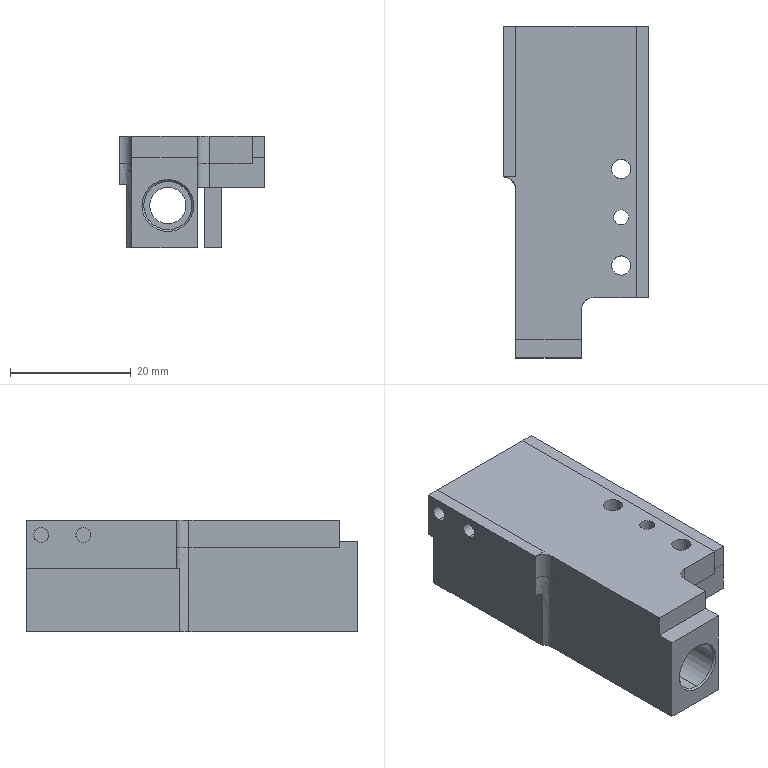NC program | NX | posted with a generic post | part box 24.15 x 55 x 18.5 mm
Lines 1748 to 2652 of 2652:
(CAVITY_MILL_COPY_COPY , TOOL : D3)
N3464 T03 M6
N3466 G54
N3468 G17 G0 G90 X18.9 Y17.954 B0. C0. S9500 M3
N3470 G43 Z30. H3
N3472 Z-0.2
N3474 G94 G1 X19. Y18.011 F1000.
N3476 G3 X19.5 Y18.877 R1.
N3478 G1 Y19.112 F1200.
N3480 G2 X20.919 Y20.573 R1.5
N3482 G1 X20.838 Y20.575
N3484 X17.928
N3486 G3 X17.062 Y20.075 R1.
N3488 G1 X17.005 Y19.975
N3490 G0 X18.9 Y17.954 Z-0.4
N3492 G1 X19. Y18.011 F1000.
N3494 G3 X19.5 Y18.877 R1.
N3496 G1 Y19.112 F1200.
N3498 G2 X20.919 Y20.573 R1.5
N3500 G1 X20.838 Y20.575
N3502 X17.928
N3504 G3 X17.062 Y20.075 R1.
N3506 G1 X17.005 Y19.975
N3508 G0 X18.9 Y17.954 Z-0.6
N3510 G1 X19. Y18.011 F1000.
N3512 G3 X19.5 Y18.877 R1.
N3514 G1 Y19.112 F1200.
N3516 G2 X20.919 Y20.573 R1.5
N3518 G1 X20.838 Y20.575
N3520 X17.928
N3522 G3 X17.062 Y20.075 R1.
N3524 G1 X17.005 Y19.975
N3526 G0 X18.9 Y17.954 Z-0.8
N3528 G1 X19. Y18.011 F1000.
N3530 G3 X19.5 Y18.877 R1.
N3532 G1 Y19.112 F1200.
N3534 G2 X20.919 Y20.573 R1.5
N3536 G1 X20.838 Y20.575
N3538 X17.928
N3540 G3 X17.062 Y20.075 R1.
N3542 G1 X17.005 Y19.975
N3544 G0 X18.9 Y17.954 Z-1.
N3546 G1 X19. Y18.011 F1000.
N3548 G3 X19.5 Y18.877 R1.
N3550 G1 Y19.112 F1200.
N3552 G2 X20.919 Y20.573 R1.5
N3554 G1 X20.838 Y20.575
N3556 X17.928
N3558 G3 X17.062 Y20.075 R1.
N3560 G1 X17.005 Y19.975
N3562 G0 X18.9 Y17.954 Z-1.2
N3564 G1 X19. Y18.011 F1000.
N3566 G3 X19.5 Y18.877 R1.
N3568 G1 Y19.112 F1200.
N3570 G2 X20.919 Y20.573 R1.5
N3572 G1 X20.838 Y20.575
N3574 X17.928
N3576 G3 X17.062 Y20.075 R1.
N3578 G1 X17.005 Y19.975
N3580 G0 X18.9 Y17.954 Z-1.4
N3582 G1 X19. Y18.011 F1000.
N3584 G3 X19.5 Y18.877 R1.
N3586 G1 Y19.112 F1200.
N3588 G2 X20.919 Y20.573 R1.5
N3590 G1 X20.838 Y20.575
N3592 X17.928
N3594 G3 X17.062 Y20.075 R1.
N3596 G1 X17.005 Y19.975
N3598 G0 X18.9 Y17.954 Z-1.6
N3600 G1 X19. Y18.011 F1000.
N3602 G3 X19.5 Y18.877 R1.
N3604 G1 Y19.112 F1200.
N3606 G2 X20.919 Y20.573 R1.5
N3608 G1 X20.838 Y20.575
N3610 X17.928
N3612 G3 X17.062 Y20.075 R1.
N3614 G1 X17.005 Y19.975
N3616 G0 X18.9 Y17.954 Z-1.8
N3618 G1 X19. Y18.011 F1000.
N3620 G3 X19.5 Y18.877 R1.
N3622 G1 Y19.112 F1200.
N3624 G2 X20.919 Y20.573 R1.5
N3626 G1 X20.838 Y20.575
N3628 X17.928
N3630 G3 X17.062 Y20.075 R1.
N3632 G1 X17.005 Y19.975
N3634 G0 X18.9 Y17.954 Z-2.
N3636 G1 X19. Y18.011 F1000.
N3638 G3 X19.5 Y18.877 R1.
N3640 G1 Y19.112 F1200.
N3642 G2 X20.919 Y20.573 R1.5
N3644 G1 X20.838 Y20.575
N3646 X17.928
N3648 G3 X17.062 Y20.075 R1.
N3650 G1 X17.005 Y19.975
N3652 G0 X18.9 Y17.954 Z-2.2
N3654 G1 X19. Y18.011 F1000.
N3656 G3 X19.5 Y18.877 R1.
N3658 G1 Y19.112 F1200.
N3660 G2 X20.919 Y20.573 R1.5
N3662 G1 X20.838 Y20.575
N3664 X17.928
N3666 G3 X17.062 Y20.075 R1.
N3668 G1 X17.005 Y19.975
N3670 G0 X18.9 Y17.954 Z-2.4
N3672 G1 X19. Y18.011 F1000.
N3674 G3 X19.5 Y18.877 R1.
N3676 G1 Y19.112 F1200.
N3678 G2 X20.919 Y20.573 R1.5
N3680 G1 X20.838 Y20.575
N3682 X17.928
N3684 G3 X17.062 Y20.075 R1.
N3686 G1 X17.005 Y19.975
N3688 G0 X18.9 Y17.954 Z-2.6
N3690 G1 X19. Y18.011 F1000.
N3692 G3 X19.5 Y18.877 R1.
N3694 G1 Y19.112 F1200.
N3696 G2 X20.919 Y20.573 R1.5
N3698 G1 X20.838 Y20.575
N3700 X17.928
N3702 G3 X17.062 Y20.075 R1.
N3704 G1 X17.005 Y19.975
N3706 G0 X18.9 Y17.954 Z-2.8
N3708 G1 X19. Y18.011 F1000.
N3710 G3 X19.5 Y18.877 R1.
N3712 G1 Y19.112 F1200.
N3714 G2 X20.919 Y20.573 R1.5
N3716 G1 X20.838 Y20.575
N3718 X17.928
N3720 G3 X17.062 Y20.075 R1.
N3722 G1 X17.005 Y19.975
N3724 G0 X18.9 Y17.954 Z-3.
N3726 G1 X19. Y18.011 F1000.
N3728 G3 X19.5 Y18.877 R1.
N3730 G1 Y19.112 F1200.
N3732 G2 X20.919 Y20.573 R1.5
N3734 G1 X20.838 Y20.575
N3736 X17.928
N3738 G3 X17.062 Y20.075 R1.
N3740 G1 X17.005 Y19.975
N3742 G0 X18.9 Y17.954 Z-3.2
N3744 G1 X19. Y18.011 F1000.
N3746 G3 X19.5 Y18.877 R1.
N3748 G1 Y19.112 F1200.
N3750 G2 X20.919 Y20.573 R1.5
N3752 G1 X20.838 Y20.575
N3754 X17.928
N3756 G3 X17.062 Y20.075 R1.
N3758 G1 X17.005 Y19.975
N3760 G0 X18.9 Y17.954 Z-3.4
N3762 G1 X19. Y18.011 F1000.
N3764 G3 X19.5 Y18.877 R1.
N3766 G1 Y19.112 F1200.
N3768 G2 X20.919 Y20.573 R1.5
N3770 G1 X20.838 Y20.575
N3772 X17.928
N3774 G3 X17.062 Y20.075 R1.
N3776 G1 X17.005 Y19.975
N3778 G0 X18.9 Y17.954 Z-3.6
N3780 G1 X19. Y18.011 F1000.
N3782 G3 X19.5 Y18.877 R1.
N3784 G1 Y19.112 F1200.
N3786 G2 X20.919 Y20.573 R1.5
N3788 G1 X20.838 Y20.575
N3790 X17.928
N3792 G3 X17.062 Y20.075 R1.
N3794 G1 X17.005 Y19.975
N3796 G0 X18.9 Y17.954 Z-3.8
N3798 G1 X19. Y18.011 F1000.
N3800 G3 X19.5 Y18.877 R1.
N3802 G1 Y19.112 F1200.
N3804 G2 X20.919 Y20.573 R1.5
N3806 G1 X20.838 Y20.575
N3808 X17.928
N3810 G3 X17.062 Y20.075 R1.
N3812 G1 X17.005 Y19.975
N3814 G0 X18.9 Y17.954 Z-4.
N3816 G1 X19. Y18.011 F1000.
N3818 G3 X19.5 Y18.877 R1.
N3820 G1 Y19.075 F1200.
N3822 G2 X20.919 Y20.573 R1.5
N3824 G1 X20.838 Y20.575
N3826 X17.928
N3828 G3 X17.062 Y20.075 R1.
N3830 G1 X17.005 Y19.975
N3832 G0 X18.9 Y17.954 Z-4.2
N3834 G1 X19. Y18.011 F1000.
N3836 G3 X19.5 Y18.877 R1.
N3838 G1 Y19.075 F1200.
N3840 G2 X20.919 Y20.573 R1.5
N3842 G1 X20.838 Y20.575
N3844 X17.928
N3846 G3 X17.062 Y20.075 R1.
N3848 G1 X17.005 Y19.975
N3850 G0 X18.9 Y17.954 Z-4.4
N3852 G1 X19. Y18.011 F1000.
N3854 G3 X19.5 Y18.877 R1.
N3856 G1 Y19.075 F1200.
N3858 G2 X20.919 Y20.573 R1.5
N3860 G1 X20.838 Y20.575
N3862 X17.928
N3864 G3 X17.062 Y20.075 R1.
N3866 G1 X17.005 Y19.975
N3868 G0 X18.9 Y17.954 Z-4.6
N3870 G1 X19. Y18.011 F1000.
N3872 G3 X19.5 Y18.877 R1.
N3874 G1 Y19.075 F1200.
N3876 G2 X20.919 Y20.573 R1.5
N3878 G1 X20.838 Y20.575
N3880 X17.928
N3882 G3 X17.062 Y20.075 R1.
N3884 G1 X17.005 Y19.975
N3886 G0 X18.9 Y17.954 Z-4.8
N3888 G1 X19. Y18.011 F1000.
N3890 G3 X19.5 Y18.877 R1.
N3892 G1 Y19.075 F1200.
N3894 G2 X20.919 Y20.573 R1.5
N3896 G1 X20.838 Y20.575
N3898 X17.928
N3900 G3 X17.062 Y20.075 R1.
N3902 G1 X17.005 Y19.975
N3904 G0 X18.9 Y17.954 Z-5.
N3906 G1 X19. Y18.011 F1000.
N3908 G3 X19.5 Y18.877 R1.
N3910 G1 Y19.075 F1200.
N3912 G2 X20.919 Y20.573 R1.5
N3914 G1 X20.838 Y20.575
N3916 X17.928
N3918 G3 X17.062 Y20.075 R1.
N3920 G1 X17.005 Y19.975
N3922 G0 X18.9 Y17.954 Z-5.2
N3924 G1 X19. Y18.011 F1000.
N3926 G3 X19.5 Y18.877 R1.
N3928 G1 Y19.075 F1200.
N3930 G2 X20.919 Y20.573 R1.5
N3932 G1 X20.838 Y20.575
N3934 X17.928
N3936 G3 X17.062 Y20.075 R1.
N3938 G1 X17.005 Y19.975
N3940 G0 X18.9 Y17.954 Z-5.4
N3942 G1 X19. Y18.011 F1000.
N3944 G3 X19.5 Y18.877 R1.
N3946 G1 Y19.075 F1200.
N3948 G2 X20.919 Y20.573 R1.5
N3950 G1 X20.838 Y20.575
N3952 X17.928
N3954 G3 X17.062 Y20.075 R1.
N3956 G1 X17.005 Y19.975
N3958 G0 X18.9 Y17.954 Z-5.6
N3960 G1 X19. Y18.011 F1000.
N3962 G3 X19.5 Y18.877 R1.
N3964 G1 Y19.075 F1200.
N3966 G2 X20.919 Y20.573 R1.5
N3968 G1 X20.838 Y20.575
N3970 X17.928
N3972 G3 X17.062 Y20.075 R1.
N3974 G1 X17.005 Y19.975
N3976 G0 X18.9 Y17.954 Z-5.8
N3978 G1 X19. Y18.011 F1000.
N3980 G3 X19.5 Y18.877 R1.
N3982 G1 Y19.075 F1200.
N3984 G2 X20.919 Y20.573 R1.5
N3986 G1 X20.838 Y20.575
N3988 X17.928
N3990 G3 X17.062 Y20.075 R1.
N3992 G1 X17.005 Y19.975
N3994 G0 X18.9 Y17.954 Z-6.
N3996 G1 X19. Y18.011 F1000.
N3998 G3 X19.5 Y18.877 R1.
N4000 G1 Y19.075 F1200.
N4002 G2 X20.919 Y20.573 R1.5
N4004 G1 X20.838 Y20.575
N4006 X17.928
N4008 G3 X17.062 Y20.075 R1.
N4010 G1 X17.005 Y19.975
N4012 G0 X18.9 Y17.954 Z-6.2
N4014 G1 X19. Y18.011 F1000.
N4016 G3 X19.5 Y18.877 R1.
N4018 G1 Y19.075 F1200.
N4020 G2 X20.919 Y20.573 R1.5
N4022 G1 X20.838 Y20.575
N4024 X17.928
N4026 G3 X17.062 Y20.075 R1.
N4028 G1 X17.005 Y19.975
N4030 G0 X18.9 Y17.954 Z-6.4
N4032 G1 X19. Y18.011 F1000.
N4034 G3 X19.5 Y18.877 R1.
N4036 G1 Y19.075 F1200.
N4038 G2 X20.919 Y20.573 R1.5
N4040 G1 X20.838 Y20.575
N4042 X17.928
N4044 G3 X17.062 Y20.075 R1.
N4046 G1 X17.005 Y19.975
N4048 G0 X18.9 Y17.954 Z-6.6
N4050 G1 X19. Y18.011 F1000.
N4052 G3 X19.5 Y18.877 R1.
N4054 G1 Y19.075 F1200.
N4056 G2 X20.919 Y20.573 R1.5
N4058 G1 X20.838 Y20.575
N4060 X17.928
N4062 G3 X17.062 Y20.075 R1.
N4064 G1 X17.005 Y19.975
N4066 G0 X18.9 Y17.954 Z-6.8
N4068 G1 X19. Y18.011 F1000.
N4070 G3 X19.5 Y18.877 R1.
N4072 G1 Y19.075 F1200.
N4074 G2 X20.919 Y20.573 R1.5
N4076 G1 X20.838 Y20.575
N4078 X17.928
N4080 G3 X17.062 Y20.075 R1.
N4082 G1 X17.005 Y19.975
N4084 G0 X18.9 Y17.954 Z-7.
N4086 G1 X19. Y18.011 F1000.
N4088 G3 X19.5 Y18.877 R1.
N4090 G1 Y19.075 F1200.
N4092 G2 X20.919 Y20.573 R1.5
N4094 G1 X20.838 Y20.575
N4096 X17.928
N4098 G3 X17.062 Y20.075 R1.
N4100 G1 X17.005 Y19.975
N4102 G0 X18.9 Y17.954 Z-7.2
N4104 G1 X19. Y18.011 F1000.
N4106 G3 X19.5 Y18.877 R1.
N4108 G1 Y19.075 F1200.
N4110 G2 X20.919 Y20.573 R1.5
N4112 G1 X20.838 Y20.575
N4114 X17.928
N4116 G3 X17.062 Y20.075 R1.
N4118 G1 X17.005 Y19.975
N4120 G0 X18.9 Y17.954 Z-7.4
N4122 G1 X19. Y18.011 F1000.
N4124 G3 X19.5 Y18.877 R1.
N4126 G1 Y19.075 F1200.
N4128 G2 X20.919 Y20.573 R1.5
N4130 G1 X20.838 Y20.575
N4132 X17.928
N4134 G3 X17.062 Y20.075 R1.
N4136 G1 X17.005 Y19.975
N4138 G0 X18.9 Y17.954 Z-7.6
N4140 G1 X19. Y18.011 F1000.
N4142 G3 X19.5 Y18.877 R1.
N4144 G1 Y19.075 F1200.
N4146 G2 X20.919 Y20.573 R1.5
N4148 G1 X20.838 Y20.575
N4150 X17.928
N4152 G3 X17.062 Y20.075 R1.
N4154 G1 X17.005 Y19.975
N4156 G0 X18.9 Y17.954 Z-7.8
N4158 G1 X19. Y18.011 F1000.
N4160 G3 X19.5 Y18.877 R1.
N4162 G1 Y19.075 F1200.
N4164 G2 X20.919 Y20.573 R1.5
N4166 G1 X20.838 Y20.575
N4168 X17.928
N4170 G3 X17.062 Y20.075 R1.
N4172 G1 X17.005 Y19.975
N4174 G0 X18.9 Y17.954 Z-8.
N4176 G1 X19. Y18.011 F1000.
N4178 G3 X19.5 Y18.877 R1.
N4180 G1 Y19.075 F1200.
N4182 G2 X20.919 Y20.573 R1.5
N4184 G1 X20.838 Y20.575
N4186 X17.928
N4188 G3 X17.062 Y20.075 R1.
N4190 G1 X17.005 Y19.975
N4192 G0 X18.9 Y17.954 Z-8.2
N4194 G1 X19. Y18.011 F1000.
N4196 G3 X19.5 Y18.877 R1.
N4198 G1 Y19.075 F1200.
N4200 G2 X20.919 Y20.573 R1.5
N4202 G1 X20.838 Y20.575
N4204 X17.928
N4206 G3 X17.062 Y20.075 R1.
N4208 G1 X17.005 Y19.975
N4210 G0 X18.9 Y17.954 Z-8.4
N4212 G1 X19. Y18.011 F1000.
N4214 G3 X19.5 Y18.877 R1.
N4216 G1 Y19.075 F1200.
N4218 G2 X20.919 Y20.573 R1.5
N4220 G1 X20.838 Y20.575
N4222 X17.928
N4224 G3 X17.062 Y20.075 R1.
N4226 G1 X17.005 Y19.975
N4228 G0 X18.9 Y17.954 Z-8.6
N4230 G1 X19. Y18.011 F1000.
N4232 G3 X19.5 Y18.877 R1.
N4234 G1 Y19.075 F1200.
N4236 G2 X20.919 Y20.573 R1.5
N4238 G1 X20.838 Y20.575
N4240 X17.928
N4242 G3 X17.062 Y20.075 R1.
N4244 G1 X17.005 Y19.975
N4246 G0 X18.9 Y17.954 Z-8.8
N4248 G1 X19. Y18.011 F1000.
N4250 G3 X19.5 Y18.877 R1.
N4252 G1 Y19.075 F1200.
N4254 G2 X20.919 Y20.573 R1.5
N4256 G1 X20.838 Y20.575
N4258 X17.928
N4260 G3 X17.062 Y20.075 R1.
N4262 G1 X17.005 Y19.975
N4264 G0 X18.9 Y17.954 Z-9.
N4266 G1 X19. Y18.011 F1000.
N4268 G3 X19.5 Y18.877 R1.
N4270 G1 Y19.075 F1200.
N4272 G2 X20.919 Y20.573 R1.5
N4274 G1 X20.838 Y20.575
N4276 X17.928
N4278 G3 X17.062 Y20.075 R1.
N4280 G1 X17.005 Y19.975
N4282 G0 X18.9 Y17.954 Z-9.2
N4284 G1 X19. Y18.011 F1000.
N4286 G3 X19.5 Y18.877 R1.
N4288 G1 Y19.075 F1200.
N4290 G2 X20.919 Y20.573 R1.5
N4292 G1 X20.838 Y20.575
N4294 X17.928
N4296 G3 X17.062 Y20.075 R1.
N4298 G1 X17.005 Y19.975
N4300 G0 X18.9 Y17.954 Z-9.4
N4302 G1 X19. Y18.011 F1000.
N4304 G3 X19.5 Y18.877 R1.
N4306 G1 Y19.075 F1200.
N4308 G2 X20.919 Y20.573 R1.5
N4310 G1 X20.838 Y20.575
N4312 X17.928
N4314 G3 X17.062 Y20.075 R1.
N4316 G1 X17.005 Y19.975
N4318 G0 X18.9 Y17.954 Z-9.6
N4320 G1 X19. Y18.011 F1000.
N4322 G3 X19.5 Y18.877 R1.
N4324 G1 Y19.075 F1200.
N4326 G2 X20.919 Y20.573 R1.5
N4328 G1 X20.838 Y20.575
N4330 X17.928
N4332 G3 X17.062 Y20.075 R1.
N4334 G1 X17.005 Y19.975
N4336 G0 X18.9 Y17.954 Z-9.8
N4338 G1 X19. Y18.011 F1000.
N4340 G3 X19.5 Y18.877 R1.
N4342 G1 Y19.075 F1200.
N4344 G2 X20.919 Y20.573 R1.5
N4346 G1 X20.838 Y20.575
N4348 X17.928
N4350 G3 X17.062 Y20.075 R1.
N4352 G1 X17.005 Y19.975
N4354 G0 X18.9 Y17.954 Z-10.
N4356 G1 X19. Y18.011 F1000.
N4358 G3 X19.5 Y18.877 R1.
N4360 G1 Y19.075 F1200.
N4362 G2 X20.919 Y20.573 R1.5
N4364 G1 X20.838 Y20.575
N4366 X17.928
N4368 G3 X17.062 Y20.075 R1.
N4370 G1 X17.005 Y19.975
N4372 G0 X18.9 Y17.954 Z-10.2
N4374 G1 X19. Y18.011 F1000.
N4376 G3 X19.5 Y18.877 R1.
N4378 G1 Y19.075 F1200.
N4380 G2 X20.919 Y20.573 R1.5
N4382 G1 X20.838 Y20.575
N4384 X17.928
N4386 G3 X17.062 Y20.075 R1.
N4388 G1 X17.005 Y19.975
N4390 G0 X18.9 Y17.954 Z-10.4
N4392 G1 X19. Y18.011 F1000.
N4394 G3 X19.5 Y18.877 R1.
N4396 G1 Y19.075 F1200.
N4398 G2 X20.919 Y20.573 R1.5
N4400 G1 X20.838 Y20.575
N4402 X17.928
N4404 G3 X17.062 Y20.075 R1.
N4406 G1 X17.005 Y19.975
N4408 G0 X18.9 Y17.954 Z-10.6
N4410 G1 X19. Y18.011 F1000.
N4412 G3 X19.5 Y18.877 R1.
N4414 G1 Y19.075 F1200.
N4416 G2 X20.879 Y20.57 R1.5
N4418 G1 X20.838 Y20.575
N4420 X17.928
N4422 G3 X17.062 Y20.075 R1.
N4424 G1 X17.005 Y19.975
N4426 G0 X18.9 Y17.954 Z-10.8
N4428 G1 X19. Y18.011 F1000.
N4430 G3 X19.5 Y18.877 R1.
N4432 G1 Y19.075 F1200.
N4434 G2 X20.879 Y20.57 R1.5
N4436 G1 X20.838 Y20.575
N4438 X17.928
N4440 G3 X17.062 Y20.075 R1.
N4442 G1 X17.005 Y19.975
N4444 G0 X18.9 Y17.954 Z-11.
N4446 G1 X19. Y18.011 F1000.
N4448 G3 X19.5 Y18.877 R1.
N4450 G1 Y19.075 F1200.
N4452 G2 X20.879 Y20.57 R1.5
N4454 G1 X20.838 Y20.575
N4456 X17.928
N4458 G3 X17.062 Y20.075 R1.
N4460 G1 X17.005 Y19.975
N4462 G0 X18.9 Y17.954 Z-11.2
N4464 G1 X19. Y18.011 F1000.
N4466 G3 X19.5 Y18.877 R1.
N4468 G1 Y19.075 F1200.
N4470 G2 X20.879 Y20.57 R1.5
N4472 G1 X20.838 Y20.575
N4474 X17.928
N4476 G3 X17.062 Y20.075 R1.
N4478 G1 X17.005 Y19.975
N4480 G0 X18.9 Y17.954 Z-11.4
N4482 G1 X19. Y18.011 F1000.
N4484 G3 X19.5 Y18.877 R1.
N4486 G1 Y19.075 F1200.
N4488 G2 X20.879 Y20.57 R1.5
N4490 G1 X20.838 Y20.575
N4492 X17.928
N4494 G3 X17.062 Y20.075 R1.
N4496 G1 X17.005 Y19.975
N4498 G0 X18.9 Y17.954 Z-11.6
N4500 G1 X19. Y18.011 F1000.
N4502 G3 X19.5 Y18.877 R1.
N4504 G1 Y19.075 F1200.
N4506 G2 X20.938 Y20.574 R1.5
N4508 G1 X20.838 Y20.575
N4510 X17.928
N4512 G3 X17.062 Y20.075 R1.
N4514 G1 X17.005 Y19.975
N4516 G0 X18.9 Y17.954 Z-11.8
N4518 G1 X19. Y18.011 F1000.
N4520 G3 X19.5 Y18.877 R1.
N4522 G1 Y19.075 F1200.
N4524 G2 X20.935 Y20.574 R1.5
N4526 G1 X20.838 Y20.575
N4528 X17.928
N4530 G3 X17.062 Y20.075 R1.
N4532 G1 X17.005 Y19.975
N4534 G0 X18.9 Y17.954 Z-12.
N4536 G1 X19. Y18.011 F1000.
N4538 G3 X19.5 Y18.877 R1.
N4540 G1 Y19.075 F1200.
N4542 G2 X20.919 Y20.573 R1.5
N4544 G1 X20.838 Y20.575
N4546 X17.928
N4548 G3 X17.062 Y20.075 R1.
N4550 G1 X17.005 Y19.975
N4552 G0 Z30.
N4554 X16.879 Y12.175
N4556 Z-10.2
N4558 G1 X16.936 Y12.075 F1000.
N4560 G3 X17.802 Y11.575 R1.
N4562 G1 X18. F1200.
N4564 G2 X19.5 Y10.075 R1.5
N4566 G1 Y13.147
N4568 G3 X19. Y14.013 R1.
N4570 G1 X18.9 Y14.07
N4572 G0 X16.879 Y12.175 Z-10.4
N4574 G1 X16.936 Y12.075 F1000.
N4576 G3 X17.802 Y11.575 R1.
N4578 G1 X18. F1200.
N4580 G2 X19.5 Y10.075 R1.5
N4582 G1 Y13.147
N4584 G3 X19. Y14.013 R1.
N4586 G1 X18.9 Y14.07
N4588 G0 X16.879 Y12.175 Z-10.6
N4590 G1 X16.936 Y12.075 F1000.
N4592 G3 X17.802 Y11.575 R1.
N4594 G1 X18. F1200.
N4596 G2 X19.5 Y10.075 R1.5
N4598 G1 Y13.147
N4600 G3 X19. Y14.013 R1.
N4602 G1 X18.9 Y14.07
N4604 G0 X16.879 Y12.175 Z-10.8
N4606 G1 X16.936 Y12.075 F1000.
N4608 G3 X17.802 Y11.575 R1.
N4610 G1 X18. F1200.
N4612 G2 X19.5 Y10.075 R1.5
N4614 G1 Y13.147
N4616 G3 X19. Y14.013 R1.
N4618 G1 X18.9 Y14.07
N4620 G0 X16.879 Y12.175 Z-11.
N4622 G1 X16.936 Y12.075 F1000.
N4624 G3 X17.802 Y11.575 R1.
N4626 G1 X18. F1200.
N4628 G2 X19.5 Y10.075 R1.5
N4630 G1 Y13.147
N4632 G3 X19. Y14.013 R1.
N4634 G1 X18.9 Y14.07
N4636 G0 X16.879 Y12.175 Z-11.2
N4638 G1 X16.936 Y12.075 F1000.
N4640 G3 X17.802 Y11.575 R1.
N4642 G1 X18. F1200.
N4644 G2 X19.5 Y10.075 R1.5
N4646 G1 Y13.147
N4648 G3 X19. Y14.013 R1.
N4650 G1 X18.9 Y14.07
N4652 G0 X16.879 Y12.175 Z-11.4
N4654 G1 X16.936 Y12.075 F1000.
N4656 G3 X17.802 Y11.575 R1.
N4658 G1 X18. F1200.
N4660 G2 X19.5 Y10.075 R1.5
N4662 G1 Y13.147
N4664 G3 X19. Y14.013 R1.
N4666 G1 X18.9 Y14.07
N4668 G0 X16.879 Y12.175 Z-11.6
N4670 G1 X16.936 Y12.075 F1000.
N4672 G3 X17.802 Y11.575 R1.
N4674 G1 X18. F1200.
N4676 G2 X19.5 Y10.075 R1.5
N4678 G1 Y13.147
N4680 G3 X19. Y14.013 R1.
N4682 G1 X18.9 Y14.07
N4684 G0 X16.879 Y12.175 Z-11.8
N4686 G1 X16.936 Y12.075 F1000.
N4688 G3 X17.802 Y11.575 R1.
N4690 G1 X18. F1200.
N4692 G2 X19.5 Y10.075 R1.5
N4694 G1 Y13.147
N4696 G3 X19. Y14.013 R1.
N4698 G1 X18.9 Y14.07
N4700 G0 X16.879 Y12.175 Z-12.
N4702 G1 X16.936 Y12.075 F1000.
N4704 G3 X17.802 Y11.575 R1.
N4706 G1 X18. F1200.
N4708 G2 X19.5 Y10.075 R1.5
N4710 G1 Y13.147
N4712 G3 X19. Y14.013 R1.
N4714 G1 X18.9 Y14.07
N4716 G0 Z30.
N4718 X-1.56 Y5.608
N4720 Z-10.2
N4722 G1 X-0.31 F1000.
N4724 G2 X-0.06 Y5.175 R0.5
N4726 G1 Y4.674 F1200.
N4728 X0. Y4.675
N4730 X13.
N4732 G3 X13. Y5.675 R0.5
N4734 G1 X0.
N4736 X-0.06 Y5.676
N4738 Y5.175
N4740 G2 X-0.31 Y4.742 R0.5
N4742 G1 X-1.56
N4744 G0 Y5.608 Z-10.4
N4746 G1 X-0.31 F1000.
N4748 G2 X-0.06 Y5.175 R0.5
N4750 G1 Y4.674 F1200.
N4752 X0. Y4.675
N4754 X13.
N4756 G3 X13. Y5.675 R0.5
N4758 G1 X0.
N4760 X-0.06 Y5.676
N4762 Y5.175
N4764 G2 X-0.31 Y4.742 R0.5
N4766 G1 X-1.56
N4768 G0 Y5.608 Z-10.6
N4770 G1 X-0.31 F1000.
N4772 G2 X-0.06 Y5.175 R0.5
N4774 G1 Y4.674 F1200.
N4776 X0. Y4.675
N4778 X13.
N4780 G3 X13. Y5.675 R0.5
N4782 G1 X0.
N4784 X-0.06 Y5.676
N4786 Y5.175
N4788 G2 X-0.31 Y4.742 R0.5
N4790 G1 X-1.56
N4792 G0 Y5.608 Z-10.8
N4794 G1 X-0.31 F1000.
N4796 G2 X-0.06 Y5.175 R0.5
N4798 G1 Y4.674 F1200.
N4800 X0. Y4.675
N4802 X13.
N4804 G3 X13. Y5.675 R0.5
N4806 G1 X0.
N4808 X-0.06 Y5.676
N4810 Y5.175
N4812 G2 X-0.31 Y4.742 R0.5
N4814 G1 X-1.56
N4816 G0 Y5.608 Z-11.
N4818 G1 X-0.31 F1000.
N4820 G2 X-0.06 Y5.175 R0.5
N4822 G1 Y4.674 F1200.
N4824 X0. Y4.675
N4826 X13.
N4828 G3 X13. Y5.675 R0.5
N4830 G1 X0.
N4832 X-0.06 Y5.676
N4834 Y5.175
N4836 G2 X-0.31 Y4.742 R0.5
N4838 G1 X-1.56
N4840 G0 Y5.608 Z-11.2
N4842 G1 X-0.31 F1000.
N4844 G2 X-0.06 Y5.175 R0.5
N4846 G1 Y4.674 F1200.
N4848 X0. Y4.675
N4850 X13.
N4852 G3 X13. Y5.675 R0.5
N4854 G1 X0.
N4856 X-0.06 Y5.676
N4858 Y5.175
N4860 G2 X-0.31 Y4.742 R0.5
N4862 G1 X-1.56
N4864 G0 Y5.608 Z-11.4
N4866 G1 X-0.31 F1000.
N4868 G2 X-0.06 Y5.175 R0.5
N4870 G1 Y4.674 F1200.
N4872 X0. Y4.675
N4874 X13.
N4876 G3 X13. Y5.675 R0.5
N4878 G1 X0.
N4880 X-0.06 Y5.676
N4882 Y5.175
N4884 G2 X-0.31 Y4.742 R0.5
N4886 G1 X-1.56
N4888 G0 Y5.608 Z-11.6
N4890 G1 X-0.31 F1000.
N4892 G2 X-0.06 Y5.175 R0.5
N4894 G1 Y4.674 F1200.
N4896 X0. Y4.675
N4898 X13.
N4900 G3 X13. Y5.675 R0.5
N4902 G1 X0.
N4904 X-0.06 Y5.676
N4906 Y5.175
N4908 G2 X-0.31 Y4.742 R0.5
N4910 G1 X-1.56
N4912 G0 Y5.608 Z-11.8
N4914 G1 X-0.31 F1000.
N4916 G2 X-0.06 Y5.175 R0.5
N4918 G1 Y4.674 F1200.
N4920 X0. Y4.675
N4922 X13.
N4924 G3 X13. Y5.675 R0.5
N4926 G1 X0.
N4928 X-0.06 Y5.676
N4930 Y5.175
N4932 G2 X-0.31 Y4.742 R0.5
N4934 G1 X-1.56
N4936 G0 Y5.608 Z-12.
N4938 G1 X-0.31 F1000.
N4940 G2 X-0.06 Y5.175 R0.5
N4942 G1 Y4.674 F1200.
N4944 X0. Y4.675
N4946 X13.
N4948 G3 X13. Y5.675 R0.5
N4950 G1 X0.
N4952 X-0.06 Y5.676
N4954 Y5.175
N4956 G2 X-0.31 Y4.742 R0.5
N4958 G1 X-1.56
N4960 G0 Z30.
N4962 M5
(PLANAR_MILL , TOOL : D6A45)
N4964 T07 M6
N4966 G54
N4968 G17 G0 G90 X38.766 Y9.868 B0. C0. S9500 M3
N4970 G43 Z30. H7
N4972 Z2.
N4974 G94 G1 Z-1. F1250.
N4976 G3 X38. Y10.225 R1.
N4978 G1 X21.
N4980 G2 X20.05 Y11.175 R0.95
N4982 G1 Y19.075
N4984 G2 X21. Y20.025 R0.95
N4986 G3 X21.55 Y20.575 R0.55
N4988 X21. Y21.125 R0.55
N4990 G1 X0.
N4992 G2 X-0.95 Y22.075 R0.95
N4994 G1 Y22.875
N4996 G2 X0. Y23.825 R0.95
N4998 G1 X25.401
N5000 G2 X26.16 Y23.446 R0.95
N5002 G3 X26.532 Y23.136 R1.056
N5004 X27. Y23.025 R1.045
N5006 G1 X55.
N5008 G2 X55.95 Y22.075 R0.95
N5010 G1 Y11.175
N5012 G2 X55. Y10.225 R0.95
N5014 G1 X38.
N5016 G3 X37.234 Y9.868 R1.
N5018 G1 Z2.
N5020 G0 Z30.
N5022 X7.266 Y5.868
N5024 Z2.
N5026 G1 Z-1.
N5028 G3 X6.5 Y6.225 R1.
N5030 G1 X0.
N5032 G2 X-0.95 Y7.175 R0.95
N5034 G1 Y10.075
N5036 G2 X0. Y11.025 R0.95
N5038 G1 X13.
N5040 G2 X13.95 Y10.075 R0.95
N5042 G1 Y7.175
N5044 G2 X13. Y6.225 R0.95
N5046 G1 X6.5
N5048 G3 X5.734 Y5.868 R1.
N5050 G1 Z2.
N5052 G0 Z30.
(PLANAR_MILL_COPY , TOOL : D6A45)
N5054 X39.297 Y3.552
N5056 Z-8.
N5058 G1 Z-11.
N5060 X38.934 Y2.632
N5062 G3 X39.7 Y2.275 R1.
N5064 X42. Y4.575 R2.3
N5066 X39.7 Y2.275 R-2.3
N5068 X40.466 Y2.632 R1.
N5070 G1 X40.103 Y3.552
N5072 Z-8.
N5074 G0 Z30.
N5076 X47.423 Y6.975
N5078 Z-8.
N5080 G1 Z-11.
N5082 X46.716 Y7.818
N5084 G3 X45.95 Y8.175 R1.
N5086 G1 Y0.05
N5088 G2 X44.95 Y-0.95 R1.
N5090 G1 X0.05
N5092 G2 X-0.95 Y0.05 R1.
N5094 G1 Y3.125
N5096 G2 X0.05 Y4.125 R1.
N5098 G1 X13.
N5100 G3 X13.391 Y4.201 R1.05
N5102 G1 Z-8.
N5104 G0 Z30.
N5106 X16.376 Y12.573
N5108 Z-8.
N5110 G1 Z-11.
N5112 X15.942 Y11.865
N5114 G3 X15.846 Y11.025 R1.
N5116 G1 X18.004 Y11.024
N5118 G3 X17.608 Y11.771 R1.
N5120 G1 X16.8 Y12.382
N5122 Z-8.
N5124 G0 Z30.
N5126 X31.791 Y4.875
N5128 Z-8.
N5130 G1 X31.563 Z-8.061
N5132 X31.4 Y4.712 Z-8.123
N5134 Y4.438 Z-8.196
N5136 X31.563 Y4.275 Z-8.258
N5138 X31.837 Z-8.332
N5140 X32. Y4.438 Z-8.393
N5142 Y4.712 Z-8.467
N5144 X31.837 Y4.875 Z-8.528
N5146 X31.563 Z-8.602
N5148 X31.4 Y4.712 Z-8.664
N5150 Y4.438 Z-8.737
N5152 X31.563 Y4.275 Z-8.799
N5154 X31.837 Z-8.873
N5156 X32. Y4.438 Z-8.934
N5158 Y4.712 Z-9.008
N5160 X31.837 Y4.875 Z-9.07
N5162 X31.563 Z-9.143
N5164 X31.4 Y4.712 Z-9.205
N5166 Y4.438 Z-9.278
N5168 X31.563 Y4.275 Z-9.34
N5170 X31.837 Z-9.414
N5172 X32. Y4.438 Z-9.475
N5174 Y4.712 Z-9.549
N5176 X31.837 Y4.875 Z-9.611
N5178 X31.563 Z-9.684
N5180 X31.4 Y4.712 Z-9.746
N5182 Y4.438 Z-9.819
N5184 X31.563 Y4.275 Z-9.881
N5186 X31.837 Z-9.955
N5188 X32. Y4.438 Z-10.016
N5190 Y4.712 Z-10.09
N5192 X31.837 Y4.875 Z-10.152
N5194 X31.563 Z-10.225
N5196 X31.4 Y4.712 Z-10.287
N5198 Y4.438 Z-10.361
N5200 X31.563 Y4.275 Z-10.422
N5202 X31.837 Z-10.496
N5204 X32. Y4.438 Z-10.557
N5206 Y4.712 Z-10.631
N5208 X31.837 Y4.875 Z-10.693
N5210 X31.563 Z-10.766
N5212 X31.4 Y4.712 Z-10.828
N5214 Y4.438 Z-10.902
N5216 X31.563 Y4.275 Z-10.963
N5218 X31.7 Z-11.
N5220 G3 X32. Y4.575 R0.3
N5222 X31.7 Y4.275 R-0.3
N5224 X31.567 Y4.676 R0.5
N5226 G1 Z-8.
N5228 G0 Z30.
N5230 X23.297 Y3.552
N5232 Z-8.
N5234 G1 Z-11.
N5236 X22.934 Y2.632
N5238 G3 X23.7 Y2.275 R1.
N5240 X26. Y4.575 R2.3
N5242 X23.7 Y2.275 R-2.3
N5244 X24.466 Y2.632 R1.
N5246 G1 X24.103 Y3.552
N5248 Z-8.
N5250 G0 Z30.
N5252 M5
N5254 M2